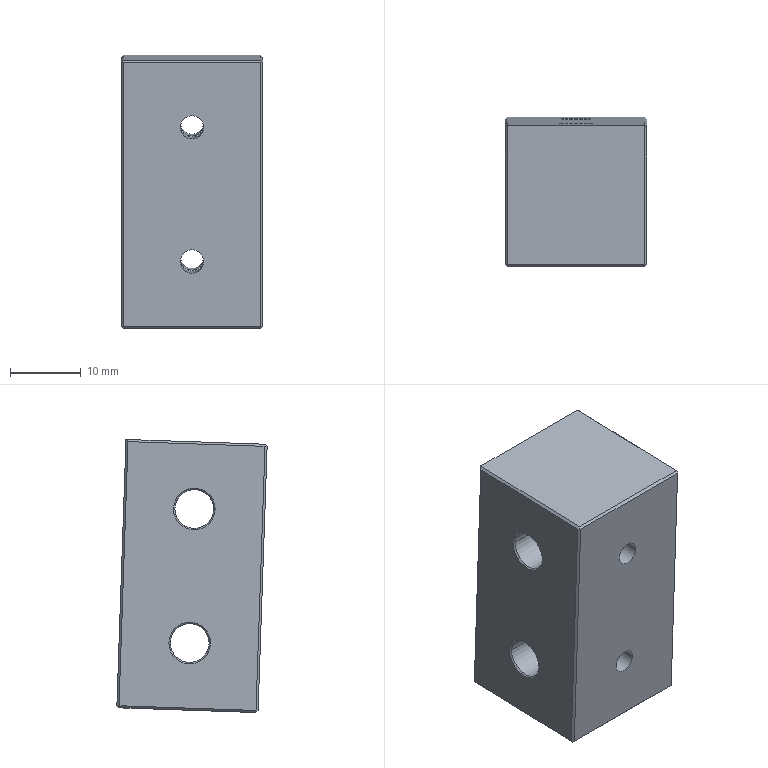Part | NX | 1 solid | 41 faces | box 20 x 21.268 x 38.652 mm | volume 13980 mm3 | plane 17 | cylinder 16 | cone 8 | commonest cylinder face diameters 3.3 x8 5.5 x8